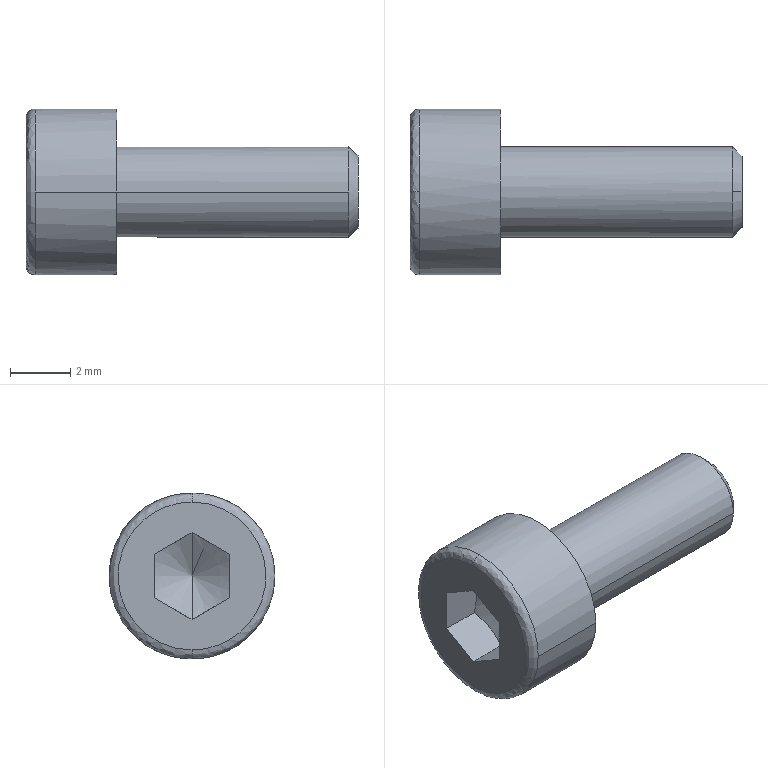Part | SolidWorks | features BaseBody 1 | 1 solid | 19 faces | box 11 x 5.5 x 5.5 mm | volume 118.284 mm3 | plane 9 | cylinder 4 | cone 4 | spline 2 | commonest cylinder face diameters 3 x2 5.5 x2
STEP:
#1=CARTESIAN_POINT('',(-2.7,0.,2.75));
#2=VERTEX_POINT('',#1);
#3=CARTESIAN_POINT('',(-2.7,-2.75,0.));
#4=VERTEX_POINT('',#3);
#5=CARTESIAN_POINT('',(-2.7,0.,0.));
#6=DIRECTION('',(1.,0.,0.));
#7=DIRECTION('',(0.,1.,0.));
#8=AXIS2_PLACEMENT_3D('',#5,#6,#7);
#9=CIRCLE('',#8,2.75);
#10=EDGE_CURVE('',#2,#4,#9,.T.);
#11=ORIENTED_EDGE('',*,*,#10,.F.);
#12=CARTESIAN_POINT('',(-3.,0.,2.45));
#13=VERTEX_POINT('',#12);
#14=CARTESIAN_POINT('',(-2.7,0.,2.45));
#15=DIRECTION('',(0.,-1.,0.));
#16=DIRECTION('',(0.,0.,1.));
#17=AXIS2_PLACEMENT_3D('',#14,#15,#16);
#18=CIRCLE('',#17,0.3);
#19=EDGE_CURVE('',#2,#13,#18,.T.);
#20=ORIENTED_EDGE('',*,*,#19,.T.);
#21=CARTESIAN_POINT('',(-3.,0.,-2.45));
#22=VERTEX_POINT('',#21);
#23=CARTESIAN_POINT('',(-3.,0.,2.45));
#24=CARTESIAN_POINT('',(-3.,-4.9,2.45));
#25=CARTESIAN_POINT('',(-3.,-4.9,-2.45));
#26=CARTESIAN_POINT('',(-3.,0.,-2.45));
#27=(BOUNDED_CURVE()B_SPLINE_CURVE(3,(#23,#24,#25,#26),.UNSPECIFIED.,.F.,.F.)B_SPLINE_CURVE_WITH_KNOTS((4,4),(0.25,0.75),.UNSPECIFIED.)CURVE()GEOMETRIC_REPRESENTATION_ITEM()RATIONAL_B_SPLINE_CURVE((1.,0.3333,0.3333,1.))REPRESENTATION_ITEM(''));
#28=EDGE_CURVE('',#13,#22,#27,.T.);
#29=ORIENTED_EDGE('',*,*,#28,.T.);
#30=CARTESIAN_POINT('',(-2.7,0.,-2.75));
#31=VERTEX_POINT('',#30);
#32=CARTESIAN_POINT('',(-2.7,0.,-2.45));
#33=DIRECTION('',(0.,1.,0.));
#34=DIRECTION('',(0.,0.,-1.));
#35=AXIS2_PLACEMENT_3D('',#32,#33,#34);
#36=CIRCLE('',#35,0.3);
#37=EDGE_CURVE('',#31,#22,#36,.T.);
#38=ORIENTED_EDGE('',*,*,#37,.F.);
#39=CARTESIAN_POINT('',(-2.7,0.,0.));
#40=DIRECTION('',(1.,0.,0.));
#41=DIRECTION('',(0.,1.,0.));
#42=AXIS2_PLACEMENT_3D('',#39,#40,#41);
#43=CIRCLE('',#42,2.75);
#44=EDGE_CURVE('',#4,#31,#43,.T.);
#45=ORIENTED_EDGE('',*,*,#44,.F.);
#46=EDGE_LOOP('',(#11,#20,#29,#38,#45));
#47=FACE_OUTER_BOUND('',#46,.T.);
#48=CARTESIAN_POINT('',(-2.7,0.,2.75));
#49=CARTESIAN_POINT('',(-2.7,-5.5,2.75));
#50=CARTESIAN_POINT('',(-2.7,-5.5,-2.75));
#51=CARTESIAN_POINT('',(-2.7,0.,-2.75));
#52=CARTESIAN_POINT('',(-2.876,0.,2.75));
#53=CARTESIAN_POINT('',(-2.876,-5.5,2.75));
#54=CARTESIAN_POINT('',(-2.876,-5.5,-2.75));
#55=CARTESIAN_POINT('',(-2.876,0.,-2.75));
#56=CARTESIAN_POINT('',(-3.,0.,2.626));
#57=CARTESIAN_POINT('',(-3.,-5.251,2.626));
#58=CARTESIAN_POINT('',(-3.,-5.251,-2.626));
#59=CARTESIAN_POINT('',(-3.,0.,-2.626));
#60=CARTESIAN_POINT('',(-3.,0.,2.45));
#61=CARTESIAN_POINT('',(-3.,-4.9,2.45));
#62=CARTESIAN_POINT('',(-3.,-4.9,-2.45));
#63=CARTESIAN_POINT('',(-3.,0.,-2.45));
#64=(BOUNDED_SURFACE()B_SPLINE_SURFACE(3,3,((#48,#49,#50,#51),(#52,#53,#54,#55),(#56,#57,#58,#59),(#60,#61,#62,#63)),.UNSPECIFIED.,.F.,.F.,.F.)B_SPLINE_SURFACE_WITH_KNOTS((4,4),(4,4),(0.,1.),(0.,1.),.UNSPECIFIED.)GEOMETRIC_REPRESENTATION_ITEM()RATIONAL_B_SPLINE_SURFACE(((1.,0.3333,0.3333,1.),(0.8047,0.2682,0.2682,0.8047),(0.8047,0.2682,0.2682,0.8047),(1.,0.3333,0.3333,1.)))REPRESENTATION_ITEM('')SURFACE());
#65=ADVANCED_FACE('',(#47),#64,.T.);
#66=CARTESIAN_POINT('',(0.,1.5,0.));
#67=VERTEX_POINT('',#66);
#68=CARTESIAN_POINT('',(0.,-1.5,0.));
#69=VERTEX_POINT('',#68);
#70=CARTESIAN_POINT('',(0.,0.,0.));
#71=DIRECTION('',(1.,0.,0.));
#72=DIRECTION('',(0.,1.,0.));
#73=AXIS2_PLACEMENT_3D('',#70,#71,#72);
#74=CIRCLE('',#73,1.5);
#75=EDGE_CURVE('',#67,#69,#74,.T.);
#76=ORIENTED_EDGE('',*,*,#75,.T.);
#77=CARTESIAN_POINT('',(7.693,-1.5,0.));
#78=VERTEX_POINT('',#77);
#79=CARTESIAN_POINT('',(4.625,-1.5,0.));
#80=DIRECTION('',(1.,0.,0.));
#81=VECTOR('',#80,1000.);
#82=LINE('',#79,#81);
#83=EDGE_CURVE('',#69,#78,#82,.T.);
#84=ORIENTED_EDGE('',*,*,#83,.T.);
#85=CARTESIAN_POINT('',(7.693,0.,1.5));
#86=VERTEX_POINT('',#85);
#87=CARTESIAN_POINT('',(7.693,0.,0.));
#88=DIRECTION('',(-1.,0.,0.));
#89=DIRECTION('',(0.,1.,0.));
#90=AXIS2_PLACEMENT_3D('',#87,#88,#89);
#91=CIRCLE('',#90,1.5);
#92=EDGE_CURVE('',#78,#86,#91,.T.);
#93=ORIENTED_EDGE('',*,*,#92,.T.);
#94=CARTESIAN_POINT('',(7.693,1.5,0.));
#95=VERTEX_POINT('',#94);
#96=CARTESIAN_POINT('',(7.693,0.,0.));
#97=DIRECTION('',(-1.,0.,0.));
#98=DIRECTION('',(0.,1.,0.));
#99=AXIS2_PLACEMENT_3D('',#96,#97,#98);
#100=CIRCLE('',#99,1.5);
#101=EDGE_CURVE('',#86,#95,#100,.T.);
#102=ORIENTED_EDGE('',*,*,#101,.T.);
#103=CARTESIAN_POINT('',(4.625,1.5,0.));
#104=DIRECTION('',(1.,0.,0.));
#105=VECTOR('',#104,1000.);
#106=LINE('',#103,#105);
#107=EDGE_CURVE('',#67,#95,#106,.T.);
#108=ORIENTED_EDGE('',*,*,#107,.F.);
#109=EDGE_LOOP('',(#76,#84,#93,#102,#108));
#110=FACE_OUTER_BOUND('',#109,.T.);
#111=CARTESIAN_POINT('',(4.625,0.,0.));
#112=DIRECTION('',(1.,0.,0.));
#113=DIRECTION('',(0.,1.,0.));
#114=AXIS2_PLACEMENT_3D('',#111,#112,#113);
#115=CYLINDRICAL_SURFACE('',#114,1.5);
#116=ADVANCED_FACE('',(#110),#115,.T.);
#117=CARTESIAN_POINT('',(8.,0.,1.193));
#118=VERTEX_POINT('',#117);
#119=CARTESIAN_POINT('',(8.,0.,-1.193));
#120=VERTEX_POINT('',#119);
#121=CARTESIAN_POINT('',(8.,0.,0.));
#122=DIRECTION('',(-1.,0.,0.));
#123=DIRECTION('',(0.,0.,1.));
#124=AXIS2_PLACEMENT_3D('',#121,#122,#123);
#125=CIRCLE('',#124,1.193);
#126=EDGE_CURVE('',#118,#120,#125,.T.);
#127=ORIENTED_EDGE('',*,*,#126,.T.);
#128=CARTESIAN_POINT('',(7.693,0.,-1.5));
#129=VERTEX_POINT('',#128);
#130=CARTESIAN_POINT('',(7.693,0.,-1.5));
#131=DIRECTION('',(-0.7071,0.,-0.7071));
#132=VECTOR('',#131,1000.);
#133=LINE('',#130,#132);
#134=EDGE_CURVE('',#120,#129,#133,.T.);
#135=ORIENTED_EDGE('',*,*,#134,.T.);
#136=CARTESIAN_POINT('',(7.693,0.,0.));
#137=DIRECTION('',(-1.,0.,0.));
#138=DIRECTION('',(0.,1.,0.));
#139=AXIS2_PLACEMENT_3D('',#136,#137,#138);
#140=CIRCLE('',#139,1.5);
#141=EDGE_CURVE('',#95,#129,#140,.T.);
#142=ORIENTED_EDGE('',*,*,#141,.F.);
#143=ORIENTED_EDGE('',*,*,#101,.F.);
#144=CARTESIAN_POINT('',(7.693,0.,1.5));
#145=DIRECTION('',(-0.7071,0.,0.7071));
#146=VECTOR('',#145,1000.);
#147=LINE('',#144,#146);
#148=EDGE_CURVE('',#118,#86,#147,.T.);
#149=ORIENTED_EDGE('',*,*,#148,.F.);
#150=EDGE_LOOP('',(#127,#135,#142,#143,#149));
#151=FACE_OUTER_BOUND('',#150,.T.);
#152=CARTESIAN_POINT('',(7.693,0.,0.));
#153=DIRECTION('',(-1.,0.,0.));
#154=DIRECTION('',(0.,0.,1.));
#155=AXIS2_PLACEMENT_3D('',#152,#153,#154);
#156=CONICAL_SURFACE('',#155,1.5,0.7854);
#157=ADVANCED_FACE('',(#151),#156,.T.);
#158=CARTESIAN_POINT('',(-2.7,2.75,0.));
#159=VERTEX_POINT('',#158);
#160=CARTESIAN_POINT('',(-2.7,0.,0.));
#161=DIRECTION('',(1.,0.,0.));
#162=DIRECTION('',(0.,1.,0.));
#163=AXIS2_PLACEMENT_3D('',#160,#161,#162);
#164=CIRCLE('',#163,2.75);
#165=EDGE_CURVE('',#159,#2,#164,.T.);
#166=ORIENTED_EDGE('',*,*,#165,.T.);
#167=ORIENTED_EDGE('',*,*,#10,.T.);
#168=CARTESIAN_POINT('',(0.,-2.75,0.));
#169=VERTEX_POINT('',#168);
#170=CARTESIAN_POINT('',(-1.5,-2.75,0.));
#171=DIRECTION('',(1.,0.,0.));
#172=VECTOR('',#171,1000.);
#173=LINE('',#170,#172);
#174=EDGE_CURVE('',#4,#169,#173,.T.);
#175=ORIENTED_EDGE('',*,*,#174,.T.);
#176=CARTESIAN_POINT('',(0.,2.75,0.));
#177=VERTEX_POINT('',#176);
#178=CARTESIAN_POINT('',(0.,0.,0.));
#179=DIRECTION('',(1.,0.,0.));
#180=DIRECTION('',(0.,1.,0.));
#181=AXIS2_PLACEMENT_3D('',#178,#179,#180);
#182=CIRCLE('',#181,2.75);
#183=EDGE_CURVE('',#177,#169,#182,.T.);
#184=ORIENTED_EDGE('',*,*,#183,.F.);
#185=CARTESIAN_POINT('',(-1.5,2.75,0.));
#186=DIRECTION('',(1.,0.,0.));
#187=VECTOR('',#186,1000.);
#188=LINE('',#185,#187);
#189=EDGE_CURVE('',#159,#177,#188,.T.);
#190=ORIENTED_EDGE('',*,*,#189,.F.);
#191=EDGE_LOOP('',(#166,#167,#175,#184,#190));
#192=FACE_OUTER_BOUND('',#191,.T.);
#193=CARTESIAN_POINT('',(-1.5,0.,0.));
#194=DIRECTION('',(1.,0.,0.));
#195=DIRECTION('',(0.,1.,0.));
#196=AXIS2_PLACEMENT_3D('',#193,#194,#195);
#197=CYLINDRICAL_SURFACE('',#196,2.75);
#198=ADVANCED_FACE('',(#192),#197,.T.);
#199=CARTESIAN_POINT('',(-0.8667,0.,0.));
#200=VERTEX_POINT('',#199);
#201=CARTESIAN_POINT('',(-1.7,0.,1.443));
#202=VERTEX_POINT('',#201);
#203=CARTESIAN_POINT('',(-1.705,0.,1.452));
#204=DIRECTION('',(-0.5,0.,0.866));
#205=VECTOR('',#204,1000.);
#206=LINE('',#203,#205);
#207=EDGE_CURVE('',#200,#202,#206,.T.);
#208=ORIENTED_EDGE('',*,*,#207,.F.);
#209=CARTESIAN_POINT('',(-1.7,0.,-1.443));
#210=VERTEX_POINT('',#209);
#211=CARTESIAN_POINT('',(-1.705,0.,-1.452));
#212=DIRECTION('',(-0.5,0.,-0.866));
#213=VECTOR('',#212,1000.);
#214=LINE('',#211,#213);
#215=EDGE_CURVE('',#200,#210,#214,.T.);
#216=ORIENTED_EDGE('',*,*,#215,.T.);
#217=CARTESIAN_POINT('',(-1.7,-1.25,-0.7217));
#218=VERTEX_POINT('',#217);
#219=CARTESIAN_POINT('',(-1.7,0.,-1.443));
#220=CARTESIAN_POINT('',(-1.632,-0.2041,-1.326));
#221=CARTESIAN_POINT('',(-1.589,-0.4113,-1.206));
#222=CARTESIAN_POINT('',(-1.588,-0.8364,-0.9605));
#223=CARTESIAN_POINT('',(-1.632,-1.046,-0.8397));
#224=CARTESIAN_POINT('',(-1.7,-1.25,-0.7217));
#225=B_SPLINE_CURVE_WITH_KNOTS('',3,(#219,#220,#221,#222,#223,#224),.UNSPECIFIED.,.F.,.F.,(4,2,4),(0.,0.0007289,0.001458),.UNSPECIFIED.);
#226=EDGE_CURVE('',#210,#218,#225,.T.);
#227=ORIENTED_EDGE('',*,*,#226,.T.);
#228=CARTESIAN_POINT('',(-1.7,-1.25,0.7217));
#229=VERTEX_POINT('',#228);
#230=CARTESIAN_POINT('',(-1.7,-1.25,-0.7217));
#231=CARTESIAN_POINT('',(-1.632,-1.25,-0.486));
#232=CARTESIAN_POINT('',(-1.589,-1.25,-0.2468));
#233=CARTESIAN_POINT('',(-1.588,-1.25,0.244));
#234=CARTESIAN_POINT('',(-1.632,-1.25,0.4857));
#235=CARTESIAN_POINT('',(-1.7,-1.25,0.7217));
#236=B_SPLINE_CURVE_WITH_KNOTS('',3,(#230,#231,#232,#233,#234,#235),.UNSPECIFIED.,.F.,.F.,(4,2,4),(0.,0.0007289,0.001458),.UNSPECIFIED.);
#237=EDGE_CURVE('',#218,#229,#236,.T.);
#238=ORIENTED_EDGE('',*,*,#237,.T.);
#239=CARTESIAN_POINT('',(-1.7,-1.25,0.7217));
#240=CARTESIAN_POINT('',(-1.632,-1.046,0.8395));
#241=CARTESIAN_POINT('',(-1.589,-0.8387,0.9591));
#242=CARTESIAN_POINT('',(-1.588,-0.4136,1.205));
#243=CARTESIAN_POINT('',(-1.632,-0.2044,1.325));
#244=CARTESIAN_POINT('',(-1.7,0.,1.443));
#245=B_SPLINE_CURVE_WITH_KNOTS('',3,(#239,#240,#241,#242,#243,#244),.UNSPECIFIED.,.F.,.F.,(4,2,4),(0.,0.0007289,0.001458),.UNSPECIFIED.);
#246=EDGE_CURVE('',#229,#202,#245,.T.);
#247=ORIENTED_EDGE('',*,*,#246,.T.);
#248=EDGE_LOOP('',(#208,#216,#227,#238,#247));
#249=FACE_OUTER_BOUND('',#248,.T.);
#250=CARTESIAN_POINT('',(-1.705,0.,0.));
#251=DIRECTION('',(-1.,0.,0.));
#252=DIRECTION('',(0.,0.,1.));
#253=AXIS2_PLACEMENT_3D('',#250,#251,#252);
#254=CONICAL_SURFACE('',#253,1.452,1.047);
#255=ADVANCED_FACE('',(#249),#254,.F.);
#256=ORIENTED_EDGE('',*,*,#83,.F.);
#257=CARTESIAN_POINT('',(0.,0.,0.));
#258=DIRECTION('',(1.,0.,0.));
#259=DIRECTION('',(0.,1.,0.));
#260=AXIS2_PLACEMENT_3D('',#257,#258,#259);
#261=CIRCLE('',#260,1.5);
#262=EDGE_CURVE('',#69,#67,#261,.T.);
#263=ORIENTED_EDGE('',*,*,#262,.T.);
#264=ORIENTED_EDGE('',*,*,#107,.T.);
#265=ORIENTED_EDGE('',*,*,#141,.T.);
#266=CARTESIAN_POINT('',(7.693,0.,0.));
#267=DIRECTION('',(-1.,0.,0.));
#268=DIRECTION('',(0.,1.,0.));
#269=AXIS2_PLACEMENT_3D('',#266,#267,#268);
#270=CIRCLE('',#269,1.5);
#271=EDGE_CURVE('',#129,#78,#270,.T.);
#272=ORIENTED_EDGE('',*,*,#271,.T.);
#273=EDGE_LOOP('',(#256,#263,#264,#265,#272));
#274=FACE_OUTER_BOUND('',#273,.T.);
#275=CARTESIAN_POINT('',(4.625,0.,0.));
#276=DIRECTION('',(1.,0.,0.));
#277=DIRECTION('',(0.,1.,0.));
#278=AXIS2_PLACEMENT_3D('',#275,#276,#277);
#279=CYLINDRICAL_SURFACE('',#278,1.5);
#280=ADVANCED_FACE('',(#274),#279,.T.);
#281=ORIENTED_EDGE('',*,*,#134,.F.);
#282=CARTESIAN_POINT('',(8.,0.,0.));
#283=DIRECTION('',(-1.,0.,0.));
#284=DIRECTION('',(0.,0.,1.));
#285=AXIS2_PLACEMENT_3D('',#282,#283,#284);
#286=CIRCLE('',#285,1.193);
#287=EDGE_CURVE('',#120,#118,#286,.T.);
#288=ORIENTED_EDGE('',*,*,#287,.T.);
#289=ORIENTED_EDGE('',*,*,#148,.T.);
#290=ORIENTED_EDGE('',*,*,#92,.F.);
#291=ORIENTED_EDGE('',*,*,#271,.F.);
#292=EDGE_LOOP('',(#281,#288,#289,#290,#291));
#293=FACE_OUTER_BOUND('',#292,.T.);
#294=CARTESIAN_POINT('',(7.693,0.,0.));
#295=DIRECTION('',(-1.,0.,0.));
#296=DIRECTION('',(0.,0.,1.));
#297=AXIS2_PLACEMENT_3D('',#294,#295,#296);
#298=CONICAL_SURFACE('',#297,1.5,0.7854);
#299=ADVANCED_FACE('',(#293),#298,.T.);
#300=ORIENTED_EDGE('',*,*,#75,.F.);
#301=ORIENTED_EDGE('',*,*,#262,.F.);
#302=EDGE_LOOP('',(#300,#301));
#303=FACE_BOUND('',#302,.T.);
#304=ORIENTED_EDGE('',*,*,#183,.T.);
#305=CARTESIAN_POINT('',(0.,0.,0.));
#306=DIRECTION('',(1.,0.,0.));
#307=DIRECTION('',(0.,1.,0.));
#308=AXIS2_PLACEMENT_3D('',#305,#306,#307);
#309=CIRCLE('',#308,2.75);
#310=EDGE_CURVE('',#169,#177,#309,.T.);
#311=ORIENTED_EDGE('',*,*,#310,.T.);
#312=EDGE_LOOP('',(#304,#311));
#313=FACE_OUTER_BOUND('',#312,.T.);
#314=CARTESIAN_POINT('',(0.,2.125,0.));
#315=DIRECTION('',(1.,0.,0.));
#316=DIRECTION('',(0.,0.,-1.));
#317=AXIS2_PLACEMENT_3D('',#314,#315,#316);
#318=PLANE('',#317);
#319=ADVANCED_FACE('',(#303,#313),#318,.T.);
#320=ORIENTED_EDGE('',*,*,#126,.F.);
#321=ORIENTED_EDGE('',*,*,#287,.F.);
#322=EDGE_LOOP('',(#320,#321));
#323=FACE_OUTER_BOUND('',#322,.T.);
#324=CARTESIAN_POINT('',(8.,0.75,0.));
#325=DIRECTION('',(1.,0.,0.));
#326=DIRECTION('',(0.,0.,-1.));
#327=AXIS2_PLACEMENT_3D('',#324,#325,#326);
#328=PLANE('',#327);
#329=ADVANCED_FACE('',(#323),#328,.T.);
#330=ORIENTED_EDGE('',*,*,#174,.F.);
#331=ORIENTED_EDGE('',*,*,#44,.T.);
#332=CARTESIAN_POINT('',(-2.7,0.,0.));
#333=DIRECTION('',(1.,0.,0.));
#334=DIRECTION('',(0.,1.,0.));
#335=AXIS2_PLACEMENT_3D('',#332,#333,#334);
#336=CIRCLE('',#335,2.75);
#337=EDGE_CURVE('',#31,#159,#336,.T.);
#338=ORIENTED_EDGE('',*,*,#337,.T.);
#339=ORIENTED_EDGE('',*,*,#189,.T.);
#340=ORIENTED_EDGE('',*,*,#310,.F.);
#341=EDGE_LOOP('',(#330,#331,#338,#339,#340));
#342=FACE_OUTER_BOUND('',#341,.T.);
#343=CARTESIAN_POINT('',(-1.5,0.,0.));
#344=DIRECTION('',(1.,0.,0.));
#345=DIRECTION('',(0.,1.,0.));
#346=AXIS2_PLACEMENT_3D('',#343,#344,#345);
#347=CYLINDRICAL_SURFACE('',#346,2.75);
#348=ADVANCED_FACE('',(#342),#347,.T.);
#349=ORIENTED_EDGE('',*,*,#19,.F.);
#350=ORIENTED_EDGE('',*,*,#165,.F.);
#351=ORIENTED_EDGE('',*,*,#337,.F.);
#352=ORIENTED_EDGE('',*,*,#37,.T.);
#353=CARTESIAN_POINT('',(-3.,0.,-2.45));
#354=CARTESIAN_POINT('',(-3.,4.9,-2.45));
#355=CARTESIAN_POINT('',(-3.,4.9,2.45));
#356=CARTESIAN_POINT('',(-3.,0.,2.45));
#357=(BOUNDED_CURVE()B_SPLINE_CURVE(3,(#353,#354,#355,#356),.UNSPECIFIED.,.F.,.F.)B_SPLINE_CURVE_WITH_KNOTS((4,4),(0.75,1.25),.UNSPECIFIED.)CURVE()GEOMETRIC_REPRESENTATION_ITEM()RATIONAL_B_SPLINE_CURVE((1.,0.3333,0.3333,1.))REPRESENTATION_ITEM(''));
#358=EDGE_CURVE('',#22,#13,#357,.T.);
#359=ORIENTED_EDGE('',*,*,#358,.T.);
#360=EDGE_LOOP('',(#349,#350,#351,#352,#359));
#361=FACE_OUTER_BOUND('',#360,.T.);
#362=CARTESIAN_POINT('',(-2.7,0.,-2.75));
#363=CARTESIAN_POINT('',(-2.7,5.5,-2.75));
#364=CARTESIAN_POINT('',(-2.7,5.5,2.75));
#365=CARTESIAN_POINT('',(-2.7,0.,2.75));
#366=CARTESIAN_POINT('',(-2.876,0.,-2.75));
#367=CARTESIAN_POINT('',(-2.876,5.5,-2.75));
#368=CARTESIAN_POINT('',(-2.876,5.5,2.75));
#369=CARTESIAN_POINT('',(-2.876,0.,2.75));
#370=CARTESIAN_POINT('',(-3.,0.,-2.626));
#371=CARTESIAN_POINT('',(-3.,5.251,-2.626));
#372=CARTESIAN_POINT('',(-3.,5.251,2.626));
#373=CARTESIAN_POINT('',(-3.,0.,2.626));
#374=CARTESIAN_POINT('',(-3.,0.,-2.45));
#375=CARTESIAN_POINT('',(-3.,4.9,-2.45));
#376=CARTESIAN_POINT('',(-3.,4.9,2.45));
#377=CARTESIAN_POINT('',(-3.,0.,2.45));
#378=(BOUNDED_SURFACE()B_SPLINE_SURFACE(3,3,((#362,#363,#364,#365),(#366,#367,#368,#369),(#370,#371,#372,#373),(#374,#375,#376,#377)),.UNSPECIFIED.,.F.,.F.,.T.)B_SPLINE_SURFACE_WITH_KNOTS((4,4),(4,4),(0.,1.),(0.,1.),.UNSPECIFIED.)GEOMETRIC_REPRESENTATION_ITEM()RATIONAL_B_SPLINE_SURFACE(((1.,0.3333,0.3333,1.),(0.8047,0.2682,0.2682,0.8047),(0.8047,0.2682,0.2682,0.8047),(1.,0.3333,0.3333,1.)))REPRESENTATION_ITEM('')SURFACE());
#379=ADVANCED_FACE('',(#361),#378,.T.);
#380=CARTESIAN_POINT('',(-3.,-1.25,-0.7217));
#381=VERTEX_POINT('',#380);
#382=CARTESIAN_POINT('',(-3.,0.,-1.443));
#383=VERTEX_POINT('',#382);
#384=CARTESIAN_POINT('',(-3.,-1.25,-0.7217));
#385=DIRECTION('',(0.,0.866,-0.5));
#386=VECTOR('',#385,1000.);
#387=LINE('',#384,#386);
#388=EDGE_CURVE('',#381,#383,#387,.T.);
#389=ORIENTED_EDGE('',*,*,#388,.T.);
#390=CARTESIAN_POINT('',(-3.,1.25,-0.7217));
#391=VERTEX_POINT('',#390);
#392=CARTESIAN_POINT('',(-3.,0.,-1.443));
#393=DIRECTION('',(0.,0.866,0.5));
#394=VECTOR('',#393,1000.);
#395=LINE('',#392,#394);
#396=EDGE_CURVE('',#383,#391,#395,.T.);
#397=ORIENTED_EDGE('',*,*,#396,.T.);
#398=CARTESIAN_POINT('',(-3.,1.25,0.7217));
#399=VERTEX_POINT('',#398);
#400=CARTESIAN_POINT('',(-3.,1.25,0.));
#401=DIRECTION('',(0.,0.,1.));
#402=VECTOR('',#401,1000.);
#403=LINE('',#400,#402);
#404=EDGE_CURVE('',#391,#399,#403,.T.);
#405=ORIENTED_EDGE('',*,*,#404,.T.);
#406=CARTESIAN_POINT('',(-3.,0.,1.443));
#407=VERTEX_POINT('',#406);
#408=CARTESIAN_POINT('',(-3.,1.25,0.7217));
#409=DIRECTION('',(0.,-0.866,0.5));
#410=VECTOR('',#409,1000.);
#411=LINE('',#408,#410);
#412=EDGE_CURVE('',#399,#407,#411,.T.);
#413=ORIENTED_EDGE('',*,*,#412,.T.);
#414=CARTESIAN_POINT('',(-3.,-1.25,0.7217));
#415=VERTEX_POINT('',#414);
#416=CARTESIAN_POINT('',(-3.,0.,1.443));
#417=DIRECTION('',(0.,-0.866,-0.5));
#418=VECTOR('',#417,1000.);
#419=LINE('',#416,#418);
#420=EDGE_CURVE('',#407,#415,#419,.T.);
#421=ORIENTED_EDGE('',*,*,#420,.T.);
#422=CARTESIAN_POINT('',(-3.,-1.25,0.));
#423=DIRECTION('',(0.,0.,-1.));
#424=VECTOR('',#423,1000.);
#425=LINE('',#422,#424);
#426=EDGE_CURVE('',#415,#381,#425,.T.);
#427=ORIENTED_EDGE('',*,*,#426,.T.);
#428=EDGE_LOOP('',(#389,#397,#405,#413,#421,#427));
#429=FACE_BOUND('',#428,.T.);
#430=ORIENTED_EDGE('',*,*,#358,.F.);
#431=ORIENTED_EDGE('',*,*,#28,.F.);
#432=EDGE_LOOP('',(#430,#431));
#433=FACE_OUTER_BOUND('',#432,.T.);
#434=CARTESIAN_POINT('',(-3.,2.097,0.));
#435=DIRECTION('',(-1.,0.,0.));
#436=DIRECTION('',(0.,0.,1.));
#437=AXIS2_PLACEMENT_3D('',#434,#435,#436);
#438=PLANE('',#437);
#439=ADVANCED_FACE('',(#429,#433),#438,.T.);
#440=CARTESIAN_POINT('',(-1.7,1.25,-0.7217));
#441=VERTEX_POINT('',#440);
#442=CARTESIAN_POINT('',(-3.,1.25,-0.7217));
#443=DIRECTION('',(1.,0.,0.));
#444=VECTOR('',#443,1000.);
#445=LINE('',#442,#444);
#446=EDGE_CURVE('',#391,#441,#445,.T.);
#447=ORIENTED_EDGE('',*,*,#446,.F.);
#448=ORIENTED_EDGE('',*,*,#396,.F.);
#449=CARTESIAN_POINT('',(-3.,0.,-1.443));
#450=DIRECTION('',(-1.,0.,0.));
#451=VECTOR('',#450,1000.);
#452=LINE('',#449,#451);
#453=EDGE_CURVE('',#210,#383,#452,.T.);
#454=ORIENTED_EDGE('',*,*,#453,.F.);
#455=CARTESIAN_POINT('',(-1.7,1.25,-0.7217));
#456=CARTESIAN_POINT('',(-1.632,1.046,-0.8395));
#457=CARTESIAN_POINT('',(-1.589,0.8387,-0.9591));
#458=CARTESIAN_POINT('',(-1.588,0.4136,-1.205));
#459=CARTESIAN_POINT('',(-1.632,0.2044,-1.325));
#460=CARTESIAN_POINT('',(-1.7,0.,-1.443));
#461=B_SPLINE_CURVE_WITH_KNOTS('',3,(#455,#456,#457,#458,#459,#460),.UNSPECIFIED.,.F.,.F.,(4,2,4),(0.,0.0007289,0.001458),.UNSPECIFIED.);
#462=EDGE_CURVE('',#441,#210,#461,.T.);
#463=ORIENTED_EDGE('',*,*,#462,.F.);
#464=EDGE_LOOP('',(#447,#448,#454,#463));
#465=FACE_OUTER_BOUND('',#464,.T.);
#466=CARTESIAN_POINT('',(-3.,1.25,-0.7217));
#467=DIRECTION('',(0.,0.5,-0.866));
#468=DIRECTION('',(0.,0.866,0.5));
#469=AXIS2_PLACEMENT_3D('',#466,#467,#468);
#470=PLANE('',#469);
#471=ADVANCED_FACE('',(#465),#470,.F.);
#472=ORIENTED_EDGE('',*,*,#453,.T.);
#473=ORIENTED_EDGE('',*,*,#388,.F.);
#474=CARTESIAN_POINT('',(-3.,-1.25,-0.7217));
#475=DIRECTION('',(-1.,0.,0.));
#476=VECTOR('',#475,1000.);
#477=LINE('',#474,#476);
#478=EDGE_CURVE('',#218,#381,#477,.T.);
#479=ORIENTED_EDGE('',*,*,#478,.F.);
#480=ORIENTED_EDGE('',*,*,#226,.F.);
#481=EDGE_LOOP('',(#472,#473,#479,#480));
#482=FACE_OUTER_BOUND('',#481,.T.);
#483=CARTESIAN_POINT('',(-3.,0.,-1.443));
#484=DIRECTION('',(0.,-0.5,-0.866));
#485=DIRECTION('',(0.,0.866,-0.5));
#486=AXIS2_PLACEMENT_3D('',#483,#484,#485);
#487=PLANE('',#486);
#488=ADVANCED_FACE('',(#482),#487,.F.);
#489=ORIENTED_EDGE('',*,*,#478,.T.);
#490=ORIENTED_EDGE('',*,*,#426,.F.);
#491=CARTESIAN_POINT('',(-3.,-1.25,0.7217));
#492=DIRECTION('',(-1.,0.,0.));
#493=VECTOR('',#492,1000.);
#494=LINE('',#491,#493);
#495=EDGE_CURVE('',#229,#415,#494,.T.);
#496=ORIENTED_EDGE('',*,*,#495,.F.);
#497=ORIENTED_EDGE('',*,*,#237,.F.);
#498=EDGE_LOOP('',(#489,#490,#496,#497));
#499=FACE_OUTER_BOUND('',#498,.T.);
#500=CARTESIAN_POINT('',(-3.,-1.25,-0.7217));
#501=DIRECTION('',(0.,-1.,0.));
#502=DIRECTION('',(0.,0.,-1.));
#503=AXIS2_PLACEMENT_3D('',#500,#501,#502);
#504=PLANE('',#503);
#505=ADVANCED_FACE('',(#499),#504,.F.);
#506=ORIENTED_EDGE('',*,*,#495,.T.);
#507=ORIENTED_EDGE('',*,*,#420,.F.);
#508=CARTESIAN_POINT('',(-3.,0.,1.443));
#509=DIRECTION('',(-1.,0.,0.));
#510=VECTOR('',#509,1000.);
#511=LINE('',#508,#510);
#512=EDGE_CURVE('',#202,#407,#511,.T.);
#513=ORIENTED_EDGE('',*,*,#512,.F.);
#514=ORIENTED_EDGE('',*,*,#246,.F.);
#515=EDGE_LOOP('',(#506,#507,#513,#514));
#516=FACE_OUTER_BOUND('',#515,.T.);
#517=CARTESIAN_POINT('',(-3.,-1.25,0.7217));
#518=DIRECTION('',(0.,-0.5,0.866));
#519=DIRECTION('',(0.,-0.866,-0.5));
#520=AXIS2_PLACEMENT_3D('',#517,#518,#519);
#521=PLANE('',#520);
#522=ADVANCED_FACE('',(#516),#521,.F.);
#523=ORIENTED_EDGE('',*,*,#512,.T.);
#524=ORIENTED_EDGE('',*,*,#412,.F.);
#525=CARTESIAN_POINT('',(-1.7,1.25,0.7217));
#526=VERTEX_POINT('',#525);
#527=CARTESIAN_POINT('',(-3.,1.25,0.7217));
#528=DIRECTION('',(-1.,0.,0.));
#529=VECTOR('',#528,1000.);
#530=LINE('',#527,#529);
#531=EDGE_CURVE('',#526,#399,#530,.T.);
#532=ORIENTED_EDGE('',*,*,#531,.F.);
#533=CARTESIAN_POINT('',(-1.7,0.,1.443));
#534=CARTESIAN_POINT('',(-1.632,0.2041,1.326));
#535=CARTESIAN_POINT('',(-1.589,0.4113,1.206));
#536=CARTESIAN_POINT('',(-1.588,0.8364,0.9605));
#537=CARTESIAN_POINT('',(-1.632,1.046,0.8397));
#538=CARTESIAN_POINT('',(-1.7,1.25,0.7217));
#539=B_SPLINE_CURVE_WITH_KNOTS('',3,(#533,#534,#535,#536,#537,#538),.UNSPECIFIED.,.F.,.F.,(4,2,4),(0.,0.0007289,0.001458),.UNSPECIFIED.);
#540=EDGE_CURVE('',#202,#526,#539,.T.);
#541=ORIENTED_EDGE('',*,*,#540,.F.);
#542=EDGE_LOOP('',(#523,#524,#532,#541));
#543=FACE_OUTER_BOUND('',#542,.T.);
#544=CARTESIAN_POINT('',(-3.,0.,1.443));
#545=DIRECTION('',(0.,0.5,0.866));
#546=DIRECTION('',(0.,-0.866,0.5));
#547=AXIS2_PLACEMENT_3D('',#544,#545,#546);
#548=PLANE('',#547);
#549=ADVANCED_FACE('',(#543),#548,.F.);
#550=ORIENTED_EDGE('',*,*,#531,.T.);
#551=ORIENTED_EDGE('',*,*,#404,.F.);
#552=ORIENTED_EDGE('',*,*,#446,.T.);
#553=CARTESIAN_POINT('',(-1.7,1.25,0.7217));
#554=CARTESIAN_POINT('',(-1.632,1.25,0.486));
#555=CARTESIAN_POINT('',(-1.589,1.25,0.2468));
#556=CARTESIAN_POINT('',(-1.588,1.25,-0.244));
#557=CARTESIAN_POINT('',(-1.632,1.25,-0.4857));
#558=CARTESIAN_POINT('',(-1.7,1.25,-0.7217));
#559=B_SPLINE_CURVE_WITH_KNOTS('',3,(#553,#554,#555,#556,#557,#558),.UNSPECIFIED.,.F.,.F.,(4,2,4),(0.,0.0007289,0.001458),.UNSPECIFIED.);
#560=EDGE_CURVE('',#526,#441,#559,.T.);
#561=ORIENTED_EDGE('',*,*,#560,.F.);
#562=EDGE_LOOP('',(#550,#551,#552,#561));
#563=FACE_OUTER_BOUND('',#562,.T.);
#564=CARTESIAN_POINT('',(-3.,1.25,0.7217));
#565=DIRECTION('',(0.,1.,0.));
#566=DIRECTION('',(0.,0.,1.));
#567=AXIS2_PLACEMENT_3D('',#564,#565,#566);
#568=PLANE('',#567);
#569=ADVANCED_FACE('',(#563),#568,.F.);
#570=ORIENTED_EDGE('',*,*,#215,.F.);
#571=ORIENTED_EDGE('',*,*,#207,.T.);
#572=ORIENTED_EDGE('',*,*,#540,.T.);
#573=ORIENTED_EDGE('',*,*,#560,.T.);
#574=ORIENTED_EDGE('',*,*,#462,.T.);
#575=EDGE_LOOP('',(#570,#571,#572,#573,#574));
#576=FACE_OUTER_BOUND('',#575,.T.);
#577=CARTESIAN_POINT('',(-1.705,0.,0.));
#578=DIRECTION('',(-1.,0.,0.));
#579=DIRECTION('',(0.,0.,1.));
#580=AXIS2_PLACEMENT_3D('',#577,#578,#579);
#581=CONICAL_SURFACE('',#580,1.452,1.047);
#582=ADVANCED_FACE('',(#576),#581,.F.);
#583=CLOSED_SHELL('',(#65,#116,#157,#198,#255,#280,#299,#319,#329,#348,#379,#439,#471,#488,#505,#522,#549,#569,#582));
#584=MANIFOLD_SOLID_BREP('',#583);
#585=CARTESIAN_POINT('',(0.,0.,0.));
#586=DIRECTION('',(0.,0.,1.));
#587=DIRECTION('',(1.,0.,0.));
#588=AXIS2_PLACEMENT_3D('',#585,#586,#587);
#589=(LENGTH_UNIT()NAMED_UNIT(*)SI_UNIT(.MILLI.,.METRE.));
#590=UNCERTAINTY_MEASURE_WITH_UNIT(LENGTH_MEASURE(0.00001),#589,'','');
#591=(NAMED_UNIT(*)PLANE_ANGLE_UNIT()SI_UNIT($,.RADIAN.));
#592=(NAMED_UNIT(*)SI_UNIT($,.STERADIAN.)SOLID_ANGLE_UNIT());
#593=(GEOMETRIC_REPRESENTATION_CONTEXT(3)GLOBAL_UNCERTAINTY_ASSIGNED_CONTEXT((#590))GLOBAL_UNIT_ASSIGNED_CONTEXT((#589,#591,#592))REPRESENTATION_CONTEXT('',''));
#594=ADVANCED_BREP_SHAPE_REPRESENTATION('',(#584,#588),#593);